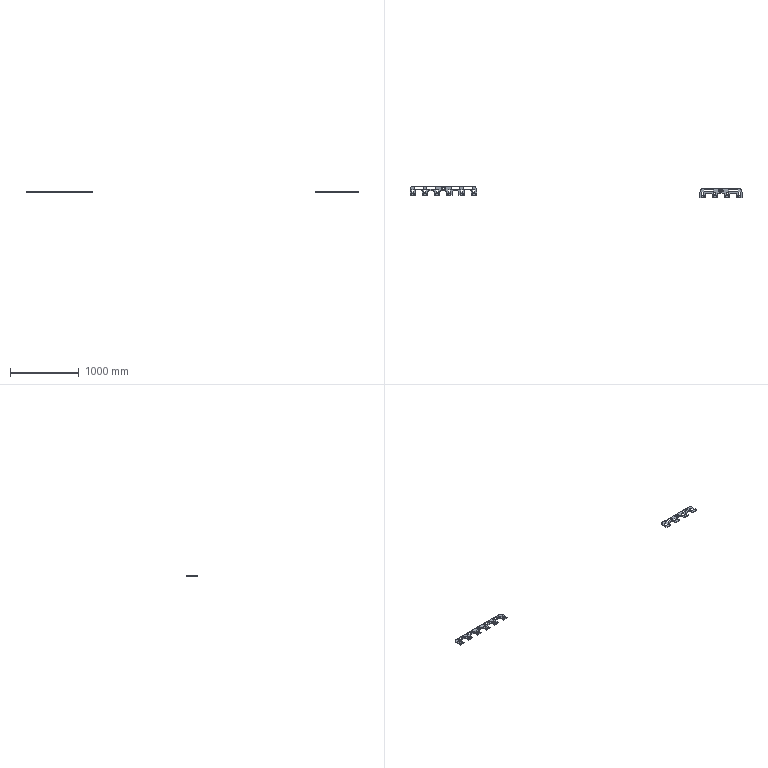NC program | NX | posted with a generic post | part box 4825 x 168.213 x 13 mm
Lines 1 to 123 of 9095:
N10 G17 G21 G94 G90
(FLOOR_WALL , TOOL : D63)
N12 T01 M6
N14 G54
N16 G17 G0 G90 X-342.1 Y68.997 S6500 M3
N18 G43 Z30. H1
N20 Z4.
N22 G94 G1 Z1. F1500.
N24 X-339.1
N26 X339.1
N28 Y40.798
N30 X-339.1
N32 Y12.599
N34 X339.1
N36 Y-15.601
N38 X-339.1
N40 Y-29.647
N42 Y-43.8
N44 X339.1
N46 X342.1
N48 Z4.
N50 G0 Z30.
N52 X-342.1 Y68.997
N54 Z3.
N56 G1 Z0.
N58 X-339.1
N60 X339.1
N62 Y40.798
N64 X-339.1
N66 Y12.599
N68 X339.1
N70 Y-15.601
N72 X-339.1
N74 Y-29.647
N76 Y-43.8
N78 X339.1
N80 X342.1
N82 Z3.
N84 G0 Z30.
N86 M5
(DRILLING , TOOL : D6A45)
N88 T07 M6
N90 G54
N92 G17 G0 G90 X-286.7 Y-39.2 S5000 M3
N94 G43 Z30. H7
N96 G94 G81 G98 Z-1. F250. R3.
N98 Y-61.2
N100 X-246.7
N102 Y-39.2
N104 X-108.9
N106 Y-61.2
N108 X-68.9
N110 Y-39.2
N112 X-10.715 Y7.131
N114 X-25.869 Y22.285
N116 X0. Y33.
N118 X-25.869 Y43.715
N120 X-10.715 Y58.869
N122 X10.715
N124 X25.869 Y43.715
N126 Y22.285
N128 X10.715 Y7.131
N130 X68.9 Y-39.2
N132 Y-61.2
N134 X108.9
N136 Y-39.2
N138 X246.7
N140 Y-61.2
N142 X286.7
N144 Y-39.2
N146 G80
N148 G0 X286.7 Y-39.2 Z30.
N150 M5
(DRILLING_COPY , TOOL : 4.5ZT)
N152 T14 M6
N154 G54
N156 G17 G0 G90 X25.869 Y22.285 S2000 M3
N158 G43 Z30. H14
N160 G94 G83 G98 Z-15.352 F250. Q2. R3.
N162 X10.715 Y7.131
N164 X-10.715
N166 X-25.869 Y22.285
N168 Y43.715
N170 X-10.715 Y58.869
N172 X10.715
N174 X25.869 Y43.715
N176 G80
N178 G0 X25.869 Y43.715 Z30.
N180 M5
(DRILLING_COPY_COPY , TOOL : 6.5ZT)
N182 T15 M6
N184 G54
N186 G17 G0 G90 X286.7 Y-39.2 S2000 M3
N188 G43 Z30. H15
N190 G94 G83 G98 Z-15.953 F250. Q2. R3.
N192 Y-61.2
N194 X246.7
N196 Y-39.2
N198 X108.9
N200 Y-61.2
N202 X68.9
N204 Y-39.2
N206 X-68.9
N208 Y-61.2
N210 X-108.9
N212 Y-39.2
N214 X-246.7
N216 Y-61.2
N218 X-286.7
N220 Y-39.2
N222 G80
N224 G0 X-286.7 Y-39.2 Z30.
N226 M5